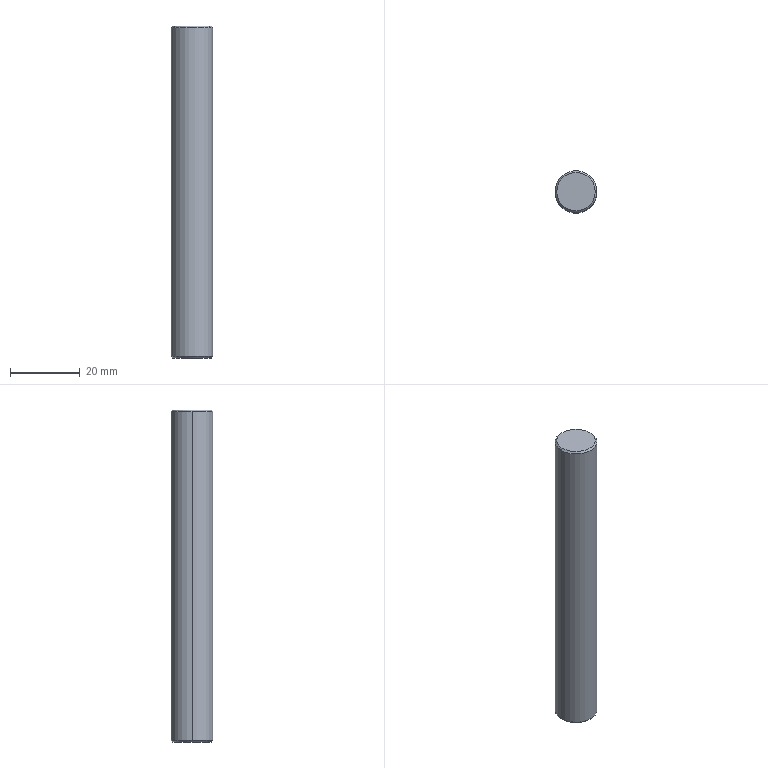Part | STEP file | PN_0024 test guide rod_Default | 1 solid | 8 faces | box 12 x 12 x 95 mm | volume 10735 mm3 | cone 4 | cylinder 2 | plane 2 | commonest cylinder face diameters 12 x2
STEP:
#1=CARTESIAN_POINT('',(0.,0.,0.));
#2=DIRECTION('',(0.,0.,1.));
#3=DIRECTION('',(1.,0.,0.));
#4=AXIS2_PLACEMENT_3D('',#1,#2,#3);
#5=CARTESIAN_POINT('',(5.5,0.,95.));
#6=VERTEX_POINT('',#5);
#7=CARTESIAN_POINT('',(-5.5,0.,95.));
#8=VERTEX_POINT('',#7);
#9=CARTESIAN_POINT('',(0.,0.,95.));
#10=DIRECTION('',(0.,0.,1.));
#11=DIRECTION('',(1.,0.,0.));
#12=AXIS2_PLACEMENT_3D('',#9,#10,#11);
#13=CIRCLE('',#12,5.5);
#14=CARTESIAN_POINT('',(0.,0.,95.));
#15=DIRECTION('',(0.,0.,-1.));
#16=DIRECTION('',(-1.,0.,0.));
#17=AXIS2_PLACEMENT_3D('',#14,#15,#16);
#18=CONICAL_SURFACE('',#17,5.5,0.7854);
#19=CARTESIAN_POINT('',(3.142,0.));
#20=DIRECTION('',(-1.,0.));
#21=VECTOR('',#20,1.);
#22=LINE('',#19,#21);
#23=(GEOMETRIC_REPRESENTATION_CONTEXT(2)PARAMETRIC_REPRESENTATION_CONTEXT()REPRESENTATION_CONTEXT('',''));
#24=DEFINITIONAL_REPRESENTATION('',(#22),#23);
#25=PCURVE('',#18,#24);
#26=CARTESIAN_POINT('',(0.,0.,95.));
#27=DIRECTION('',(0.,0.,1.));
#28=DIRECTION('',(1.,0.,0.));
#29=AXIS2_PLACEMENT_3D('',#26,#27,#28);
#30=PLANE('',#29);
#31=CARTESIAN_POINT('',(0.,0.));
#32=DIRECTION('',(1.,0.));
#33=AXIS2_PLACEMENT_2D('',#31,#32);
#34=CIRCLE('',#33,5.5);
#35=(GEOMETRIC_REPRESENTATION_CONTEXT(2)PARAMETRIC_REPRESENTATION_CONTEXT()REPRESENTATION_CONTEXT('',''));
#36=DEFINITIONAL_REPRESENTATION('',(#34),#35);
#37=PCURVE('',#30,#36);
#38=SURFACE_CURVE('',#13,(#25,#37),.PCURVE_S1.);
#39=EDGE_CURVE('',#6,#8,#38,.T.);
#40=ORIENTED_EDGE('',*,*,#39,.F.);
#41=CARTESIAN_POINT('',(6.,0.,94.5));
#42=VERTEX_POINT('',#41);
#43=CARTESIAN_POINT('',(5.5,0.,95.));
#44=DIRECTION('',(0.7071,0.,-0.7071));
#45=VECTOR('',#44,1.);
#46=LINE('',#43,#45);
#47=CARTESIAN_POINT('',(3.142,0.));
#48=DIRECTION('',(0.,1.));
#49=VECTOR('',#48,1.);
#50=LINE('',#47,#49);
#51=(GEOMETRIC_REPRESENTATION_CONTEXT(2)PARAMETRIC_REPRESENTATION_CONTEXT()REPRESENTATION_CONTEXT('',''));
#52=DEFINITIONAL_REPRESENTATION('',(#50),#51);
#53=PCURVE('',#18,#52);
#54=CARTESIAN_POINT('',(0.,0.,95.));
#55=DIRECTION('',(0.,0.,-1.));
#56=DIRECTION('',(-1.,0.,0.));
#57=AXIS2_PLACEMENT_3D('',#54,#55,#56);
#58=CONICAL_SURFACE('',#57,5.5,0.7854);
#59=CARTESIAN_POINT('',(3.142,0.));
#60=DIRECTION('',(0.,1.));
#61=VECTOR('',#60,1.);
#62=LINE('',#59,#61);
#63=(GEOMETRIC_REPRESENTATION_CONTEXT(2)PARAMETRIC_REPRESENTATION_CONTEXT()REPRESENTATION_CONTEXT('',''));
#64=DEFINITIONAL_REPRESENTATION('',(#62),#63);
#65=PCURVE('',#58,#64);
#66=SURFACE_CURVE('',#46,(#53,#65),.PCURVE_S1.);
#67=EDGE_CURVE('',#6,#42,#66,.T.);
#68=ORIENTED_EDGE('',*,*,#67,.T.);
#69=CARTESIAN_POINT('',(-6.,0.,94.5));
#70=VERTEX_POINT('',#69);
#71=CARTESIAN_POINT('',(0.,0.,94.5));
#72=DIRECTION('',(0.,0.,-1.));
#73=DIRECTION('',(1.,0.,0.));
#74=AXIS2_PLACEMENT_3D('',#71,#72,#73);
#75=CIRCLE('',#74,6.);
#76=CARTESIAN_POINT('',(-3.142,0.5));
#77=DIRECTION('',(1.,0.));
#78=VECTOR('',#77,1.);
#79=LINE('',#76,#78);
#80=(GEOMETRIC_REPRESENTATION_CONTEXT(2)PARAMETRIC_REPRESENTATION_CONTEXT()REPRESENTATION_CONTEXT('',''));
#81=DEFINITIONAL_REPRESENTATION('',(#79),#80);
#82=PCURVE('',#18,#81);
#83=CARTESIAN_POINT('',(0.,0.,95.));
#84=DIRECTION('',(0.,0.,-1.));
#85=DIRECTION('',(-1.,0.,0.));
#86=AXIS2_PLACEMENT_3D('',#83,#84,#85);
#87=CYLINDRICAL_SURFACE('',#86,6.);
#88=CARTESIAN_POINT('',(-3.142,0.5));
#89=DIRECTION('',(1.,0.));
#90=VECTOR('',#89,1.);
#91=LINE('',#88,#90);
#92=(GEOMETRIC_REPRESENTATION_CONTEXT(2)PARAMETRIC_REPRESENTATION_CONTEXT()REPRESENTATION_CONTEXT('',''));
#93=DEFINITIONAL_REPRESENTATION('',(#91),#92);
#94=PCURVE('',#87,#93);
#95=SURFACE_CURVE('',#75,(#82,#94),.PCURVE_S1.);
#96=EDGE_CURVE('',#70,#42,#95,.T.);
#97=ORIENTED_EDGE('',*,*,#96,.F.);
#98=CARTESIAN_POINT('',(-5.5,0.,95.));
#99=DIRECTION('',(-0.7071,0.,-0.7071));
#100=VECTOR('',#99,1.);
#101=LINE('',#98,#100);
#102=CARTESIAN_POINT('',(0.,0.));
#103=DIRECTION('',(0.,1.));
#104=VECTOR('',#103,1.);
#105=LINE('',#102,#104);
#106=(GEOMETRIC_REPRESENTATION_CONTEXT(2)PARAMETRIC_REPRESENTATION_CONTEXT()REPRESENTATION_CONTEXT('',''));
#107=DEFINITIONAL_REPRESENTATION('',(#105),#106);
#108=PCURVE('',#18,#107);
#109=CARTESIAN_POINT('',(6.283,0.));
#110=DIRECTION('',(0.,1.));
#111=VECTOR('',#110,1.);
#112=LINE('',#109,#111);
#113=(GEOMETRIC_REPRESENTATION_CONTEXT(2)PARAMETRIC_REPRESENTATION_CONTEXT()REPRESENTATION_CONTEXT('',''));
#114=DEFINITIONAL_REPRESENTATION('',(#112),#113);
#115=PCURVE('',#58,#114);
#116=SURFACE_CURVE('',#101,(#108,#115),.PCURVE_S1.);
#117=EDGE_CURVE('',#8,#70,#116,.T.);
#118=ORIENTED_EDGE('',*,*,#117,.F.);
#119=EDGE_LOOP('',(#40,#68,#97,#118));
#120=FACE_BOUND('',#119,.T.);
#121=ADVANCED_FACE('',(#120),#18,.T.);
#122=CARTESIAN_POINT('',(-5.5,0.,0.));
#123=VERTEX_POINT('',#122);
#124=CARTESIAN_POINT('',(5.5,0.,0.));
#125=VERTEX_POINT('',#124);
#126=CARTESIAN_POINT('',(0.,0.,0.));
#127=DIRECTION('',(0.,0.,-1.));
#128=DIRECTION('',(1.,0.,0.));
#129=AXIS2_PLACEMENT_3D('',#126,#127,#128);
#130=CIRCLE('',#129,5.5);
#131=CARTESIAN_POINT('',(0.,0.,0.5));
#132=DIRECTION('',(0.,0.,1.));
#133=DIRECTION('',(1.,0.,0.));
#134=AXIS2_PLACEMENT_3D('',#131,#132,#133);
#135=CONICAL_SURFACE('',#134,6.,0.7854);
#136=CARTESIAN_POINT('',(6.283,-0.5));
#137=DIRECTION('',(-1.,0.));
#138=VECTOR('',#137,1.);
#139=LINE('',#136,#138);
#140=(GEOMETRIC_REPRESENTATION_CONTEXT(2)PARAMETRIC_REPRESENTATION_CONTEXT()REPRESENTATION_CONTEXT('',''));
#141=DEFINITIONAL_REPRESENTATION('',(#139),#140);
#142=PCURVE('',#135,#141);
#143=CARTESIAN_POINT('',(0.,0.,0.));
#144=DIRECTION('',(0.,0.,1.));
#145=DIRECTION('',(1.,0.,0.));
#146=AXIS2_PLACEMENT_3D('',#143,#144,#145);
#147=PLANE('',#146);
#148=CARTESIAN_POINT('',(5.5,0.));
#149=CARTESIAN_POINT('',(5.5,-9.526));
#150=CARTESIAN_POINT('',(-2.75,-4.763));
#151=CARTESIAN_POINT('',(-11.,0.));
#152=CARTESIAN_POINT('',(-2.75,4.763));
#153=CARTESIAN_POINT('',(5.5,9.526));
#154=CARTESIAN_POINT('',(5.5,0.));
#155=(BOUNDED_CURVE()B_SPLINE_CURVE(2,(#148,#149,#150,#151,#152,#153,#154),.UNSPECIFIED.,.T.,.F.)B_SPLINE_CURVE_WITH_KNOTS((1,2,2,2,2,1),(-2.094,0.,2.094,4.189,6.283,8.378),.UNSPECIFIED.)CURVE()GEOMETRIC_REPRESENTATION_ITEM()RATIONAL_B_SPLINE_CURVE((1.,0.5,1.,0.5,1.,0.5,1.))REPRESENTATION_ITEM(''));
#156=(GEOMETRIC_REPRESENTATION_CONTEXT(2)PARAMETRIC_REPRESENTATION_CONTEXT()REPRESENTATION_CONTEXT('',''));
#157=DEFINITIONAL_REPRESENTATION('',(#155),#156);
#158=PCURVE('',#147,#157);
#159=SURFACE_CURVE('',#130,(#142,#158),.PCURVE_S1.);
#160=EDGE_CURVE('',#123,#125,#159,.T.);
#161=ORIENTED_EDGE('',*,*,#160,.F.);
#162=CARTESIAN_POINT('',(-6.,0.,0.5));
#163=VERTEX_POINT('',#162);
#164=CARTESIAN_POINT('',(-6.,0.,0.5));
#165=DIRECTION('',(-0.7071,0.,0.7071));
#166=VECTOR('',#165,1.);
#167=LINE('',#164,#166);
#168=CARTESIAN_POINT('',(3.142,0.));
#169=DIRECTION('',(0.,1.));
#170=VECTOR('',#169,1.);
#171=LINE('',#168,#170);
#172=(GEOMETRIC_REPRESENTATION_CONTEXT(2)PARAMETRIC_REPRESENTATION_CONTEXT()REPRESENTATION_CONTEXT('',''));
#173=DEFINITIONAL_REPRESENTATION('',(#171),#172);
#174=PCURVE('',#135,#173);
#175=CARTESIAN_POINT('',(0.,0.,0.5));
#176=DIRECTION('',(0.,0.,1.));
#177=DIRECTION('',(1.,0.,0.));
#178=AXIS2_PLACEMENT_3D('',#175,#176,#177);
#179=CONICAL_SURFACE('',#178,6.,0.7854);
#180=CARTESIAN_POINT('',(3.142,0.));
#181=DIRECTION('',(0.,1.));
#182=VECTOR('',#181,1.);
#183=LINE('',#180,#182);
#184=(GEOMETRIC_REPRESENTATION_CONTEXT(2)PARAMETRIC_REPRESENTATION_CONTEXT()REPRESENTATION_CONTEXT('',''));
#185=DEFINITIONAL_REPRESENTATION('',(#183),#184);
#186=PCURVE('',#179,#185);
#187=SURFACE_CURVE('',#167,(#174,#186),.PCURVE_S1.);
#188=EDGE_CURVE('',#123,#163,#187,.T.);
#189=ORIENTED_EDGE('',*,*,#188,.T.);
#190=CARTESIAN_POINT('',(6.,0.,0.5));
#191=VERTEX_POINT('',#190);
#192=CARTESIAN_POINT('',(0.,0.,0.5));
#193=DIRECTION('',(0.,0.,1.));
#194=DIRECTION('',(1.,0.,0.));
#195=AXIS2_PLACEMENT_3D('',#192,#193,#194);
#196=CIRCLE('',#195,6.);
#197=CARTESIAN_POINT('',(0.,0.));
#198=DIRECTION('',(1.,0.));
#199=VECTOR('',#198,1.);
#200=LINE('',#197,#199);
#201=(GEOMETRIC_REPRESENTATION_CONTEXT(2)PARAMETRIC_REPRESENTATION_CONTEXT()REPRESENTATION_CONTEXT('',''));
#202=DEFINITIONAL_REPRESENTATION('',(#200),#201);
#203=PCURVE('',#135,#202);
#204=CARTESIAN_POINT('',(3.142,94.5));
#205=DIRECTION('',(-1.,0.));
#206=VECTOR('',#205,1.);
#207=LINE('',#204,#206);
#208=(GEOMETRIC_REPRESENTATION_CONTEXT(2)PARAMETRIC_REPRESENTATION_CONTEXT()REPRESENTATION_CONTEXT('',''));
#209=DEFINITIONAL_REPRESENTATION('',(#207),#208);
#210=PCURVE('',#87,#209);
#211=SURFACE_CURVE('',#196,(#203,#210),.PCURVE_S1.);
#212=EDGE_CURVE('',#191,#163,#211,.T.);
#213=ORIENTED_EDGE('',*,*,#212,.F.);
#214=CARTESIAN_POINT('',(6.,0.,0.5));
#215=DIRECTION('',(0.7071,0.,0.7071));
#216=VECTOR('',#215,1.);
#217=LINE('',#214,#216);
#218=CARTESIAN_POINT('',(0.,0.));
#219=DIRECTION('',(0.,1.));
#220=VECTOR('',#219,1.);
#221=LINE('',#218,#220);
#222=(GEOMETRIC_REPRESENTATION_CONTEXT(2)PARAMETRIC_REPRESENTATION_CONTEXT()REPRESENTATION_CONTEXT('',''));
#223=DEFINITIONAL_REPRESENTATION('',(#221),#222);
#224=PCURVE('',#135,#223);
#225=CARTESIAN_POINT('',(6.283,0.));
#226=DIRECTION('',(0.,1.));
#227=VECTOR('',#226,1.);
#228=LINE('',#225,#227);
#229=(GEOMETRIC_REPRESENTATION_CONTEXT(2)PARAMETRIC_REPRESENTATION_CONTEXT()REPRESENTATION_CONTEXT('',''));
#230=DEFINITIONAL_REPRESENTATION('',(#228),#229);
#231=PCURVE('',#179,#230);
#232=SURFACE_CURVE('',#217,(#224,#231),.PCURVE_S1.);
#233=EDGE_CURVE('',#125,#191,#232,.T.);
#234=ORIENTED_EDGE('',*,*,#233,.F.);
#235=EDGE_LOOP('',(#161,#189,#213,#234));
#236=FACE_BOUND('',#235,.T.);
#237=ADVANCED_FACE('',(#236),#135,.T.);
#238=ORIENTED_EDGE('',*,*,#96,.T.);
#239=CARTESIAN_POINT('',(6.,0.,95.));
#240=DIRECTION('',(0.,0.,-1.));
#241=VECTOR('',#240,1.);
#242=LINE('',#239,#241);
#243=CARTESIAN_POINT('',(3.142,0.));
#244=DIRECTION('',(0.,1.));
#245=VECTOR('',#244,1.);
#246=LINE('',#243,#245);
#247=(GEOMETRIC_REPRESENTATION_CONTEXT(2)PARAMETRIC_REPRESENTATION_CONTEXT()REPRESENTATION_CONTEXT('',''));
#248=DEFINITIONAL_REPRESENTATION('',(#246),#247);
#249=PCURVE('',#87,#248);
#250=CARTESIAN_POINT('',(0.,0.,95.));
#251=DIRECTION('',(0.,0.,-1.));
#252=DIRECTION('',(-1.,0.,0.));
#253=AXIS2_PLACEMENT_3D('',#250,#251,#252);
#254=CYLINDRICAL_SURFACE('',#253,6.);
#255=CARTESIAN_POINT('',(3.142,0.));
#256=DIRECTION('',(0.,1.));
#257=VECTOR('',#256,1.);
#258=LINE('',#255,#257);
#259=(GEOMETRIC_REPRESENTATION_CONTEXT(2)PARAMETRIC_REPRESENTATION_CONTEXT()REPRESENTATION_CONTEXT('',''));
#260=DEFINITIONAL_REPRESENTATION('',(#258),#259);
#261=PCURVE('',#254,#260);
#262=SURFACE_CURVE('',#242,(#249,#261),.PCURVE_S1.);
#263=EDGE_CURVE('',#42,#191,#262,.T.);
#264=ORIENTED_EDGE('',*,*,#263,.T.);
#265=ORIENTED_EDGE('',*,*,#212,.T.);
#266=CARTESIAN_POINT('',(-6.,0.,95.));
#267=DIRECTION('',(0.,0.,-1.));
#268=VECTOR('',#267,1.);
#269=LINE('',#266,#268);
#270=CARTESIAN_POINT('',(0.,0.));
#271=DIRECTION('',(0.,1.));
#272=VECTOR('',#271,1.);
#273=LINE('',#270,#272);
#274=(GEOMETRIC_REPRESENTATION_CONTEXT(2)PARAMETRIC_REPRESENTATION_CONTEXT()REPRESENTATION_CONTEXT('',''));
#275=DEFINITIONAL_REPRESENTATION('',(#273),#274);
#276=PCURVE('',#87,#275);
#277=CARTESIAN_POINT('',(6.283,0.));
#278=DIRECTION('',(0.,1.));
#279=VECTOR('',#278,1.);
#280=LINE('',#277,#279);
#281=(GEOMETRIC_REPRESENTATION_CONTEXT(2)PARAMETRIC_REPRESENTATION_CONTEXT()REPRESENTATION_CONTEXT('',''));
#282=DEFINITIONAL_REPRESENTATION('',(#280),#281);
#283=PCURVE('',#254,#282);
#284=SURFACE_CURVE('',#269,(#276,#283),.PCURVE_S1.);
#285=EDGE_CURVE('',#70,#163,#284,.T.);
#286=ORIENTED_EDGE('',*,*,#285,.F.);
#287=EDGE_LOOP('',(#238,#264,#265,#286));
#288=FACE_BOUND('',#287,.T.);
#289=ADVANCED_FACE('',(#288),#87,.T.);
#290=ORIENTED_EDGE('',*,*,#263,.F.);
#291=CARTESIAN_POINT('',(0.,0.,94.5));
#292=DIRECTION('',(0.,0.,-1.));
#293=DIRECTION('',(1.,0.,0.));
#294=AXIS2_PLACEMENT_3D('',#291,#292,#293);
#295=CIRCLE('',#294,6.);
#296=CARTESIAN_POINT('',(3.142,0.5));
#297=DIRECTION('',(1.,0.));
#298=VECTOR('',#297,1.);
#299=LINE('',#296,#298);
#300=(GEOMETRIC_REPRESENTATION_CONTEXT(2)PARAMETRIC_REPRESENTATION_CONTEXT()REPRESENTATION_CONTEXT('',''));
#301=DEFINITIONAL_REPRESENTATION('',(#299),#300);
#302=PCURVE('',#254,#301);
#303=CARTESIAN_POINT('',(3.142,0.5));
#304=DIRECTION('',(1.,0.));
#305=VECTOR('',#304,1.);
#306=LINE('',#303,#305);
#307=(GEOMETRIC_REPRESENTATION_CONTEXT(2)PARAMETRIC_REPRESENTATION_CONTEXT()REPRESENTATION_CONTEXT('',''));
#308=DEFINITIONAL_REPRESENTATION('',(#306),#307);
#309=PCURVE('',#58,#308);
#310=SURFACE_CURVE('',#295,(#302,#309),.PCURVE_S1.);
#311=EDGE_CURVE('',#42,#70,#310,.T.);
#312=ORIENTED_EDGE('',*,*,#311,.T.);
#313=ORIENTED_EDGE('',*,*,#285,.T.);
#314=CARTESIAN_POINT('',(0.,0.,0.5));
#315=DIRECTION('',(0.,0.,1.));
#316=DIRECTION('',(1.,0.,0.));
#317=AXIS2_PLACEMENT_3D('',#314,#315,#316);
#318=CIRCLE('',#317,6.);
#319=CARTESIAN_POINT('',(9.425,94.5));
#320=DIRECTION('',(-1.,0.));
#321=VECTOR('',#320,1.);
#322=LINE('',#319,#321);
#323=(GEOMETRIC_REPRESENTATION_CONTEXT(2)PARAMETRIC_REPRESENTATION_CONTEXT()REPRESENTATION_CONTEXT('',''));
#324=DEFINITIONAL_REPRESENTATION('',(#322),#323);
#325=PCURVE('',#254,#324);
#326=CARTESIAN_POINT('',(0.,0.));
#327=DIRECTION('',(1.,0.));
#328=VECTOR('',#327,1.);
#329=LINE('',#326,#328);
#330=(GEOMETRIC_REPRESENTATION_CONTEXT(2)PARAMETRIC_REPRESENTATION_CONTEXT()REPRESENTATION_CONTEXT('',''));
#331=DEFINITIONAL_REPRESENTATION('',(#329),#330);
#332=PCURVE('',#179,#331);
#333=SURFACE_CURVE('',#318,(#325,#332),.PCURVE_S1.);
#334=EDGE_CURVE('',#163,#191,#333,.T.);
#335=ORIENTED_EDGE('',*,*,#334,.T.);
#336=EDGE_LOOP('',(#290,#312,#313,#335));
#337=FACE_BOUND('',#336,.T.);
#338=ADVANCED_FACE('',(#337),#254,.T.);
#339=CARTESIAN_POINT('',(0.,0.,95.));
#340=DIRECTION('',(0.,0.,1.));
#341=DIRECTION('',(1.,0.,0.));
#342=AXIS2_PLACEMENT_3D('',#339,#340,#341);
#343=CIRCLE('',#342,5.5);
#344=CARTESIAN_POINT('',(0.,0.));
#345=DIRECTION('',(1.,0.));
#346=AXIS2_PLACEMENT_2D('',#344,#345);
#347=CIRCLE('',#346,5.5);
#348=(GEOMETRIC_REPRESENTATION_CONTEXT(2)PARAMETRIC_REPRESENTATION_CONTEXT()REPRESENTATION_CONTEXT('',''));
#349=DEFINITIONAL_REPRESENTATION('',(#347),#348);
#350=PCURVE('',#30,#349);
#351=CARTESIAN_POINT('',(9.425,0.));
#352=DIRECTION('',(-1.,0.));
#353=VECTOR('',#352,1.);
#354=LINE('',#351,#353);
#355=(GEOMETRIC_REPRESENTATION_CONTEXT(2)PARAMETRIC_REPRESENTATION_CONTEXT()REPRESENTATION_CONTEXT('',''));
#356=DEFINITIONAL_REPRESENTATION('',(#354),#355);
#357=PCURVE('',#58,#356);
#358=SURFACE_CURVE('',#343,(#350,#357),.PCURVE_S1.);
#359=EDGE_CURVE('',#8,#6,#358,.T.);
#360=ORIENTED_EDGE('',*,*,#359,.T.);
#361=ORIENTED_EDGE('',*,*,#39,.T.);
#362=EDGE_LOOP('',(#360,#361));
#363=FACE_BOUND('',#362,.T.);
#364=ADVANCED_FACE('',(#363),#30,.T.);
#365=CARTESIAN_POINT('',(0.,0.,0.));
#366=DIRECTION('',(0.,0.,-1.));
#367=DIRECTION('',(1.,0.,0.));
#368=AXIS2_PLACEMENT_3D('',#365,#366,#367);
#369=CIRCLE('',#368,5.5);
#370=CARTESIAN_POINT('',(5.5,0.));
#371=CARTESIAN_POINT('',(5.5,-9.526));
#372=CARTESIAN_POINT('',(-2.75,-4.763));
#373=CARTESIAN_POINT('',(-11.,0.));
#374=CARTESIAN_POINT('',(-2.75,4.763));
#375=CARTESIAN_POINT('',(5.5,9.526));
#376=CARTESIAN_POINT('',(5.5,0.));
#377=(BOUNDED_CURVE()B_SPLINE_CURVE(2,(#370,#371,#372,#373,#374,#375,#376),.UNSPECIFIED.,.T.,.F.)B_SPLINE_CURVE_WITH_KNOTS((1,2,2,2,2,1),(-2.094,0.,2.094,4.189,6.283,8.378),.UNSPECIFIED.)CURVE()GEOMETRIC_REPRESENTATION_ITEM()RATIONAL_B_SPLINE_CURVE((1.,0.5,1.,0.5,1.,0.5,1.))REPRESENTATION_ITEM(''));
#378=(GEOMETRIC_REPRESENTATION_CONTEXT(2)PARAMETRIC_REPRESENTATION_CONTEXT()REPRESENTATION_CONTEXT('',''));
#379=DEFINITIONAL_REPRESENTATION('',(#377),#378);
#380=PCURVE('',#147,#379);
#381=CARTESIAN_POINT('',(6.283,-0.5));
#382=DIRECTION('',(-1.,0.));
#383=VECTOR('',#382,1.);
#384=LINE('',#381,#383);
#385=(GEOMETRIC_REPRESENTATION_CONTEXT(2)PARAMETRIC_REPRESENTATION_CONTEXT()REPRESENTATION_CONTEXT('',''));
#386=DEFINITIONAL_REPRESENTATION('',(#384),#385);
#387=PCURVE('',#179,#386);
#388=SURFACE_CURVE('',#369,(#380,#387),.PCURVE_S1.);
#389=EDGE_CURVE('',#125,#123,#388,.T.);
#390=ORIENTED_EDGE('',*,*,#389,.T.);
#391=ORIENTED_EDGE('',*,*,#160,.T.);
#392=EDGE_LOOP('',(#390,#391));
#393=FACE_BOUND('',#392,.T.);
#394=ADVANCED_FACE('',(#393),#147,.F.);
#395=ORIENTED_EDGE('',*,*,#188,.F.);
#396=ORIENTED_EDGE('',*,*,#389,.F.);
#397=ORIENTED_EDGE('',*,*,#233,.T.);
#398=ORIENTED_EDGE('',*,*,#334,.F.);
#399=EDGE_LOOP('',(#395,#396,#397,#398));
#400=FACE_BOUND('',#399,.T.);
#401=ADVANCED_FACE('',(#400),#179,.T.);
#402=ORIENTED_EDGE('',*,*,#67,.F.);
#403=ORIENTED_EDGE('',*,*,#359,.F.);
#404=ORIENTED_EDGE('',*,*,#117,.T.);
#405=ORIENTED_EDGE('',*,*,#311,.F.);
#406=EDGE_LOOP('',(#402,#403,#404,#405));
#407=FACE_BOUND('',#406,.T.);
#408=ADVANCED_FACE('',(#407),#58,.T.);
#409=CLOSED_SHELL('',(#121,#237,#289,#338,#364,#394,#401,#408));
#410=MANIFOLD_SOLID_BREP('',#409);
#411=(LENGTH_UNIT()NAMED_UNIT(*)SI_UNIT(.MILLI.,.METRE.));
#412=UNCERTAINTY_MEASURE_WITH_UNIT(LENGTH_MEASURE(0.0000001),#411,'','');
#413=(NAMED_UNIT(*)PLANE_ANGLE_UNIT()SI_UNIT($,.RADIAN.));
#414=(NAMED_UNIT(*)SI_UNIT($,.STERADIAN.)SOLID_ANGLE_UNIT());
#415=(GEOMETRIC_REPRESENTATION_CONTEXT(3)GLOBAL_UNCERTAINTY_ASSIGNED_CONTEXT((#412))GLOBAL_UNIT_ASSIGNED_CONTEXT((#411,#413,#414))REPRESENTATION_CONTEXT('',''));
#416=ADVANCED_BREP_SHAPE_REPRESENTATION('',(#4,#410),#415);